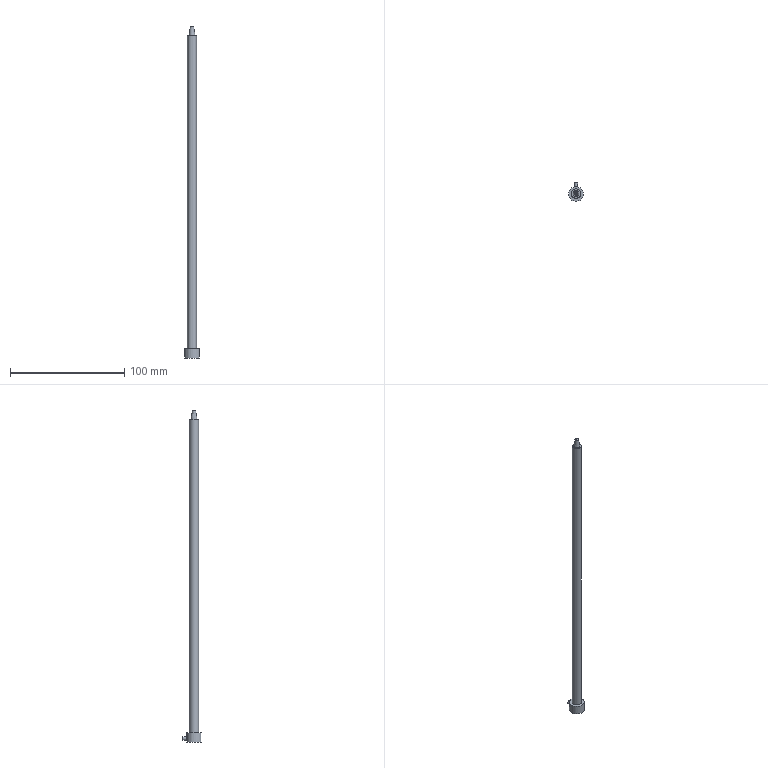Part | STEP file | E108-1-312 | 1 solid | 11 faces | box 13 x 16.5 x 290 mm | volume 14963 mm3 | plane 5 | cylinder 3 | cone 2 | spline 1 | commonest cylinder face diameters 3 x1 8 x1 13 x1
STEP:
#1=CARTESIAN_POINT('',(0.,0.,0.));
#2=DIRECTION('',(0.,0.,1.));
#3=DIRECTION('',(1.,0.,0.));
#4=AXIS2_PLACEMENT_3D('',#1,#2,#3);
#5=CARTESIAN_POINT('',(-4.,0.,282.));
#6=VERTEX_POINT('',#5);
#7=CARTESIAN_POINT('',(4.,0.,282.));
#8=VERTEX_POINT('',#7);
#9=CARTESIAN_POINT('',(0.,0.,282.));
#10=DIRECTION('',(0.,0.,1.));
#11=DIRECTION('',(1.,0.,0.));
#12=AXIS2_PLACEMENT_3D('',#9,#10,#11);
#13=CIRCLE('',#12,4.);
#14=CARTESIAN_POINT('',(0.,0.,100.));
#15=DIRECTION('',(0.,0.,-1.));
#16=DIRECTION('',(-1.,0.,0.));
#17=AXIS2_PLACEMENT_3D('',#14,#15,#16);
#18=CYLINDRICAL_SURFACE('',#17,4.);
#19=CARTESIAN_POINT('',(9.425,-182.));
#20=DIRECTION('',(-1.,0.));
#21=VECTOR('',#20,1.);
#22=LINE('',#19,#21);
#23=(GEOMETRIC_REPRESENTATION_CONTEXT(2)PARAMETRIC_REPRESENTATION_CONTEXT()REPRESENTATION_CONTEXT('',''));
#24=DEFINITIONAL_REPRESENTATION('',(#22),#23);
#25=PCURVE('',#18,#24);
#26=CARTESIAN_POINT('',(0.,0.,282.));
#27=DIRECTION('',(0.,0.,1.));
#28=DIRECTION('',(1.,0.,0.));
#29=AXIS2_PLACEMENT_3D('',#26,#27,#28);
#30=PLANE('',#29);
#31=CARTESIAN_POINT('',(0.,0.));
#32=DIRECTION('',(1.,0.));
#33=AXIS2_PLACEMENT_2D('',#31,#32);
#34=CIRCLE('',#33,4.);
#35=(GEOMETRIC_REPRESENTATION_CONTEXT(2)PARAMETRIC_REPRESENTATION_CONTEXT()REPRESENTATION_CONTEXT('',''));
#36=DEFINITIONAL_REPRESENTATION('',(#34),#35);
#37=PCURVE('',#30,#36);
#38=SURFACE_CURVE('',#13,(#25,#37),.PCURVE_S1.);
#39=EDGE_CURVE('',#6,#8,#38,.T.);
#40=ORIENTED_EDGE('',*,*,#39,.F.);
#41=CARTESIAN_POINT('',(-4.,0.,8.));
#42=VERTEX_POINT('',#41);
#43=CARTESIAN_POINT('',(-4.,0.,282.));
#44=CARTESIAN_POINT('',(-4.,0.,8.));
#45=B_SPLINE_CURVE_WITH_KNOTS('',1,(#43,#44),.UNSPECIFIED.,.F.,.F.,(2,2),(-182.,92.),.PIECEWISE_BEZIER_KNOTS.);
#46=CARTESIAN_POINT('',(6.283,0.));
#47=DIRECTION('',(0.,1.));
#48=VECTOR('',#47,1.);
#49=LINE('',#46,#48);
#50=(GEOMETRIC_REPRESENTATION_CONTEXT(2)PARAMETRIC_REPRESENTATION_CONTEXT()REPRESENTATION_CONTEXT('',''));
#51=DEFINITIONAL_REPRESENTATION('',(#49),#50);
#52=PCURVE('',#18,#51);
#53=CARTESIAN_POINT('',(0.,0.));
#54=DIRECTION('',(0.,1.));
#55=VECTOR('',#54,1.);
#56=LINE('',#53,#55);
#57=(GEOMETRIC_REPRESENTATION_CONTEXT(2)PARAMETRIC_REPRESENTATION_CONTEXT()REPRESENTATION_CONTEXT('',''));
#58=DEFINITIONAL_REPRESENTATION('',(#56),#57);
#59=PCURVE('',#18,#58);
#60=SEAM_CURVE('',#45,(#52,#59),.PCURVE_S1.);
#61=EDGE_CURVE('',#6,#42,#60,.T.);
#62=ORIENTED_EDGE('',*,*,#61,.T.);
#63=CARTESIAN_POINT('',(0.,0.,8.));
#64=DIRECTION('',(0.,0.,1.));
#65=DIRECTION('',(-1.,0.,0.));
#66=AXIS2_PLACEMENT_3D('',#63,#64,#65);
#67=CIRCLE('',#66,4.);
#68=CARTESIAN_POINT('',(6.283,92.));
#69=DIRECTION('',(-1.,0.));
#70=VECTOR('',#69,1.);
#71=LINE('',#68,#70);
#72=(GEOMETRIC_REPRESENTATION_CONTEXT(2)PARAMETRIC_REPRESENTATION_CONTEXT()REPRESENTATION_CONTEXT('',''));
#73=DEFINITIONAL_REPRESENTATION('',(#71),#72);
#74=PCURVE('',#18,#73);
#75=CARTESIAN_POINT('',(0.,0.,8.));
#76=DIRECTION('',(0.,0.,-1.));
#77=DIRECTION('',(1.,0.,0.));
#78=AXIS2_PLACEMENT_3D('',#75,#76,#77);
#79=PLANE('',#78);
#80=CARTESIAN_POINT('',(-4.,0.));
#81=CARTESIAN_POINT('',(-4.,6.928));
#82=CARTESIAN_POINT('',(2.,3.464));
#83=CARTESIAN_POINT('',(8.,0.));
#84=CARTESIAN_POINT('',(2.,-3.464));
#85=CARTESIAN_POINT('',(-4.,-6.928));
#86=CARTESIAN_POINT('',(-4.,0.));
#87=(BOUNDED_CURVE()B_SPLINE_CURVE(2,(#80,#81,#82,#83,#84,#85,#86),.UNSPECIFIED.,.T.,.F.)B_SPLINE_CURVE_WITH_KNOTS((1,2,2,2,2,1),(-2.094,0.,2.094,4.189,6.283,8.378),.UNSPECIFIED.)CURVE()GEOMETRIC_REPRESENTATION_ITEM()RATIONAL_B_SPLINE_CURVE((1.,0.5,1.,0.5,1.,0.5,1.))REPRESENTATION_ITEM(''));
#88=(GEOMETRIC_REPRESENTATION_CONTEXT(2)PARAMETRIC_REPRESENTATION_CONTEXT()REPRESENTATION_CONTEXT('',''));
#89=DEFINITIONAL_REPRESENTATION('',(#87),#88);
#90=PCURVE('',#79,#89);
#91=SURFACE_CURVE('',#67,(#74,#90),.PCURVE_S1.);
#92=EDGE_CURVE('',#42,#42,#91,.T.);
#93=ORIENTED_EDGE('',*,*,#92,.T.);
#94=ORIENTED_EDGE('',*,*,#61,.F.);
#95=CARTESIAN_POINT('',(0.,0.,282.));
#96=DIRECTION('',(0.,0.,1.));
#97=DIRECTION('',(1.,0.,0.));
#98=AXIS2_PLACEMENT_3D('',#95,#96,#97);
#99=CIRCLE('',#98,4.);
#100=CARTESIAN_POINT('',(3.142,-182.));
#101=DIRECTION('',(-1.,0.));
#102=VECTOR('',#101,1.);
#103=LINE('',#100,#102);
#104=(GEOMETRIC_REPRESENTATION_CONTEXT(2)PARAMETRIC_REPRESENTATION_CONTEXT()REPRESENTATION_CONTEXT('',''));
#105=DEFINITIONAL_REPRESENTATION('',(#103),#104);
#106=PCURVE('',#18,#105);
#107=CARTESIAN_POINT('',(0.,0.));
#108=DIRECTION('',(1.,0.));
#109=AXIS2_PLACEMENT_2D('',#107,#108);
#110=CIRCLE('',#109,4.);
#111=(GEOMETRIC_REPRESENTATION_CONTEXT(2)PARAMETRIC_REPRESENTATION_CONTEXT()REPRESENTATION_CONTEXT('',''));
#112=DEFINITIONAL_REPRESENTATION('',(#110),#111);
#113=PCURVE('',#30,#112);
#114=SURFACE_CURVE('',#99,(#106,#113),.PCURVE_S1.);
#115=EDGE_CURVE('',#8,#6,#114,.T.);
#116=ORIENTED_EDGE('',*,*,#115,.F.);
#117=EDGE_LOOP('',(#40,#62,#93,#94,#116));
#118=FACE_BOUND('',#117,.T.);
#119=ADVANCED_FACE('',(#118),#18,.T.);
#120=CARTESIAN_POINT('',(2.553,0.,282.));
#121=VERTEX_POINT('',#120);
#122=CARTESIAN_POINT('',(0.,0.,282.));
#123=DIRECTION('',(0.,0.,1.));
#124=DIRECTION('',(1.,0.,0.));
#125=AXIS2_PLACEMENT_3D('',#122,#123,#124);
#126=CIRCLE('',#125,2.553);
#127=CARTESIAN_POINT('',(0.,0.));
#128=DIRECTION('',(1.,0.));
#129=AXIS2_PLACEMENT_2D('',#127,#128);
#130=CIRCLE('',#129,2.553);
#131=(GEOMETRIC_REPRESENTATION_CONTEXT(2)PARAMETRIC_REPRESENTATION_CONTEXT()REPRESENTATION_CONTEXT('',''));
#132=DEFINITIONAL_REPRESENTATION('',(#130),#131);
#133=PCURVE('',#30,#132);
#134=CARTESIAN_POINT('',(0.,0.,290.));
#135=DIRECTION('',(0.,0.,-1.));
#136=DIRECTION('',(1.,0.,0.));
#137=AXIS2_PLACEMENT_3D('',#134,#135,#136);
#138=CONICAL_SURFACE('',#137,1.5,0.1309);
#139=CARTESIAN_POINT('',(6.283,8.));
#140=DIRECTION('',(-1.,0.));
#141=VECTOR('',#140,1.);
#142=LINE('',#139,#141);
#143=(GEOMETRIC_REPRESENTATION_CONTEXT(2)PARAMETRIC_REPRESENTATION_CONTEXT()REPRESENTATION_CONTEXT('',''));
#144=DEFINITIONAL_REPRESENTATION('',(#142),#143);
#145=PCURVE('',#138,#144);
#146=SURFACE_CURVE('',#126,(#133,#145),.PCURVE_S1.);
#147=EDGE_CURVE('',#121,#121,#146,.T.);
#148=ORIENTED_EDGE('',*,*,#147,.F.);
#149=EDGE_LOOP('',(#148));
#150=FACE_BOUND('',#149,.T.);
#151=ORIENTED_EDGE('',*,*,#115,.T.);
#152=ORIENTED_EDGE('',*,*,#39,.T.);
#153=EDGE_LOOP('',(#151,#152));
#154=FACE_BOUND('',#153,.T.);
#155=ADVANCED_FACE('',(#150,#154),#30,.T.);
#156=CARTESIAN_POINT('',(6.5,0.,0.));
#157=VERTEX_POINT('',#156);
#158=CARTESIAN_POINT('',(-6.5,0.,0.));
#159=VERTEX_POINT('',#158);
#160=CARTESIAN_POINT('',(0.,0.,0.));
#161=DIRECTION('',(0.,0.,-1.));
#162=DIRECTION('',(-1.,0.,0.));
#163=AXIS2_PLACEMENT_3D('',#160,#161,#162);
#164=CIRCLE('',#163,6.5);
#165=CARTESIAN_POINT('',(0.,0.,8.));
#166=DIRECTION('',(0.,0.,-1.));
#167=DIRECTION('',(1.,0.,0.));
#168=AXIS2_PLACEMENT_3D('',#165,#166,#167);
#169=CYLINDRICAL_SURFACE('',#168,6.5);
#170=CARTESIAN_POINT('',(-3.142,8.));
#171=DIRECTION('',(1.,0.));
#172=VECTOR('',#171,1.);
#173=LINE('',#170,#172);
#174=(GEOMETRIC_REPRESENTATION_CONTEXT(2)PARAMETRIC_REPRESENTATION_CONTEXT()REPRESENTATION_CONTEXT('',''));
#175=DEFINITIONAL_REPRESENTATION('',(#173),#174);
#176=PCURVE('',#169,#175);
#177=CARTESIAN_POINT('',(240.,-1000.,0.));
#178=DIRECTION('',(0.,0.,1.));
#179=DIRECTION('',(-1.,0.,0.));
#180=AXIS2_PLACEMENT_3D('',#177,#178,#179);
#181=PLANE('',#180);
#182=CARTESIAN_POINT('',(246.5,-1000.));
#183=CARTESIAN_POINT('',(246.5,-1011.258));
#184=CARTESIAN_POINT('',(236.75,-1005.629));
#185=CARTESIAN_POINT('',(227.,-1000.));
#186=CARTESIAN_POINT('',(236.75,-994.371));
#187=CARTESIAN_POINT('',(246.5,-988.742));
#188=CARTESIAN_POINT('',(246.5,-1000.));
#189=(BOUNDED_CURVE()B_SPLINE_CURVE(2,(#182,#183,#184,#185,#186,#187,#188),.UNSPECIFIED.,.T.,.F.)B_SPLINE_CURVE_WITH_KNOTS((1,2,2,2,2,1),(-2.094,0.,2.094,4.189,6.283,8.378),.UNSPECIFIED.)CURVE()GEOMETRIC_REPRESENTATION_ITEM()RATIONAL_B_SPLINE_CURVE((1.,0.5,1.,0.5,1.,0.5,1.))REPRESENTATION_ITEM(''));
#190=(GEOMETRIC_REPRESENTATION_CONTEXT(2)PARAMETRIC_REPRESENTATION_CONTEXT()REPRESENTATION_CONTEXT('',''));
#191=DEFINITIONAL_REPRESENTATION('',(#189),#190);
#192=PCURVE('',#181,#191);
#193=SURFACE_CURVE('',#164,(#176,#192),.PCURVE_S1.);
#194=EDGE_CURVE('',#157,#159,#193,.T.);
#195=ORIENTED_EDGE('',*,*,#194,.F.);
#196=CARTESIAN_POINT('',(6.5,0.,8.));
#197=VERTEX_POINT('',#196);
#198=CARTESIAN_POINT('',(6.5,0.,8.));
#199=CARTESIAN_POINT('',(6.5,0.,0.));
#200=B_SPLINE_CURVE_WITH_KNOTS('',1,(#198,#199),.UNSPECIFIED.,.F.,.F.,(2,2),(0.,8.),.PIECEWISE_BEZIER_KNOTS.);
#201=CARTESIAN_POINT('',(0.,0.));
#202=DIRECTION('',(0.,1.));
#203=VECTOR('',#202,1.);
#204=LINE('',#201,#203);
#205=(GEOMETRIC_REPRESENTATION_CONTEXT(2)PARAMETRIC_REPRESENTATION_CONTEXT()REPRESENTATION_CONTEXT('',''));
#206=DEFINITIONAL_REPRESENTATION('',(#204),#205);
#207=PCURVE('',#169,#206);
#208=CARTESIAN_POINT('',(6.283,0.));
#209=DIRECTION('',(0.,1.));
#210=VECTOR('',#209,1.);
#211=LINE('',#208,#210);
#212=(GEOMETRIC_REPRESENTATION_CONTEXT(2)PARAMETRIC_REPRESENTATION_CONTEXT()REPRESENTATION_CONTEXT('',''));
#213=DEFINITIONAL_REPRESENTATION('',(#211),#212);
#214=PCURVE('',#169,#213);
#215=SEAM_CURVE('',#200,(#207,#214),.PCURVE_S1.);
#216=EDGE_CURVE('',#197,#157,#215,.T.);
#217=ORIENTED_EDGE('',*,*,#216,.F.);
#218=CARTESIAN_POINT('',(0.,0.,8.));
#219=DIRECTION('',(0.,0.,-1.));
#220=DIRECTION('',(1.,0.,0.));
#221=AXIS2_PLACEMENT_3D('',#218,#219,#220);
#222=CIRCLE('',#221,6.5);
#223=CARTESIAN_POINT('',(0.,0.));
#224=DIRECTION('',(1.,0.));
#225=VECTOR('',#224,1.);
#226=LINE('',#223,#225);
#227=(GEOMETRIC_REPRESENTATION_CONTEXT(2)PARAMETRIC_REPRESENTATION_CONTEXT()REPRESENTATION_CONTEXT('',''));
#228=DEFINITIONAL_REPRESENTATION('',(#226),#227);
#229=PCURVE('',#169,#228);
#230=CARTESIAN_POINT('',(0.,0.));
#231=DIRECTION('',(1.,0.));
#232=AXIS2_PLACEMENT_2D('',#230,#231);
#233=CIRCLE('',#232,6.5);
#234=(GEOMETRIC_REPRESENTATION_CONTEXT(2)PARAMETRIC_REPRESENTATION_CONTEXT()REPRESENTATION_CONTEXT('',''));
#235=DEFINITIONAL_REPRESENTATION('',(#233),#234);
#236=PCURVE('',#79,#235);
#237=SURFACE_CURVE('',#222,(#229,#236),.PCURVE_S1.);
#238=EDGE_CURVE('',#197,#197,#237,.T.);
#239=ORIENTED_EDGE('',*,*,#238,.T.);
#240=ORIENTED_EDGE('',*,*,#216,.T.);
#241=CARTESIAN_POINT('',(0.,0.,0.));
#242=DIRECTION('',(0.,0.,-1.));
#243=DIRECTION('',(-1.,0.,0.));
#244=AXIS2_PLACEMENT_3D('',#241,#242,#243);
#245=CIRCLE('',#244,6.5);
#246=CARTESIAN_POINT('',(3.142,8.));
#247=DIRECTION('',(1.,0.));
#248=VECTOR('',#247,1.);
#249=LINE('',#246,#248);
#250=(GEOMETRIC_REPRESENTATION_CONTEXT(2)PARAMETRIC_REPRESENTATION_CONTEXT()REPRESENTATION_CONTEXT('',''));
#251=DEFINITIONAL_REPRESENTATION('',(#249),#250);
#252=PCURVE('',#169,#251);
#253=CARTESIAN_POINT('',(246.5,-1000.));
#254=CARTESIAN_POINT('',(246.5,-1011.258));
#255=CARTESIAN_POINT('',(236.75,-1005.629));
#256=CARTESIAN_POINT('',(227.,-1000.));
#257=CARTESIAN_POINT('',(236.75,-994.371));
#258=CARTESIAN_POINT('',(246.5,-988.742));
#259=CARTESIAN_POINT('',(246.5,-1000.));
#260=(BOUNDED_CURVE()B_SPLINE_CURVE(2,(#253,#254,#255,#256,#257,#258,#259),.UNSPECIFIED.,.T.,.F.)B_SPLINE_CURVE_WITH_KNOTS((1,2,2,2,2,1),(-2.094,0.,2.094,4.189,6.283,8.378),.UNSPECIFIED.)CURVE()GEOMETRIC_REPRESENTATION_ITEM()RATIONAL_B_SPLINE_CURVE((1.,0.5,1.,0.5,1.,0.5,1.))REPRESENTATION_ITEM(''));
#261=(GEOMETRIC_REPRESENTATION_CONTEXT(2)PARAMETRIC_REPRESENTATION_CONTEXT()REPRESENTATION_CONTEXT('',''));
#262=DEFINITIONAL_REPRESENTATION('',(#260),#261);
#263=PCURVE('',#181,#262);
#264=SURFACE_CURVE('',#245,(#252,#263),.PCURVE_S1.);
#265=EDGE_CURVE('',#159,#157,#264,.T.);
#266=ORIENTED_EDGE('',*,*,#265,.F.);
#267=EDGE_LOOP('',(#195,#217,#239,#240,#266));
#268=FACE_BOUND('',#267,.T.);
#269=CARTESIAN_POINT('',(0.,6.5,1.5));
#270=VERTEX_POINT('',#269);
#271=CARTESIAN_POINT('',(0.,6.5,1.5));
#272=CARTESIAN_POINT('',(0.1654,6.5,1.5));
#273=CARTESIAN_POINT('',(0.3332,6.493,1.528));
#274=CARTESIAN_POINT('',(0.4892,6.482,1.582));
#275=CARTESIAN_POINT('',(0.6451,6.47,1.636));
#276=CARTESIAN_POINT('',(0.7936,6.453,1.717));
#277=CARTESIAN_POINT('',(0.9231,6.434,1.818));
#278=CARTESIAN_POINT('',(1.055,6.415,1.92));
#279=CARTESIAN_POINT('',(1.17,6.394,2.047));
#280=CARTESIAN_POINT('',(1.261,6.377,2.187));
#281=CARTESIAN_POINT('',(1.352,6.358,2.329));
#282=CARTESIAN_POINT('',(1.421,6.343,2.49));
#283=CARTESIAN_POINT('',(1.46,6.334,2.655));
#284=CARTESIAN_POINT('',(1.498,6.325,2.817));
#285=CARTESIAN_POINT('',(1.509,6.322,2.989));
#286=CARTESIAN_POINT('',(1.492,6.326,3.155));
#287=CARTESIAN_POINT('',(1.475,6.33,3.318));
#288=CARTESIAN_POINT('',(1.431,6.341,3.48));
#289=CARTESIAN_POINT('',(1.362,6.356,3.628));
#290=CARTESIAN_POINT('',(1.293,6.37,3.777));
#291=CARTESIAN_POINT('',(1.199,6.39,3.917));
#292=CARTESIAN_POINT('',(1.085,6.409,4.035));
#293=CARTESIAN_POINT('',(0.9695,6.428,4.157));
#294=CARTESIAN_POINT('',(0.8309,6.448,4.26));
#295=CARTESIAN_POINT('',(0.6809,6.464,4.337));
#296=CARTESIAN_POINT('',(0.5305,6.48,4.413));
#297=CARTESIAN_POINT('',(0.3642,6.492,4.465));
#298=CARTESIAN_POINT('',(0.1962,6.497,4.487));
#299=CARTESIAN_POINT('',(0.03191,6.502,4.509));
#300=CARTESIAN_POINT('',(-0.1386,6.501,4.503));
#301=CARTESIAN_POINT('',(-0.3008,6.493,4.47));
#302=CARTESIAN_POINT('',(-0.4611,6.486,4.437));
#303=CARTESIAN_POINT('',(-0.6177,6.472,4.377));
#304=CARTESIAN_POINT('',(-0.7583,6.456,4.294));
#305=CARTESIAN_POINT('',(-0.9011,6.439,4.211));
#306=CARTESIAN_POINT('',(-1.031,6.419,4.102));
#307=CARTESIAN_POINT('',(-1.139,6.399,3.976));
#308=CARTESIAN_POINT('',(-1.249,6.38,3.848));
#309=CARTESIAN_POINT('',(-1.338,6.361,3.699));
#310=CARTESIAN_POINT('',(-1.399,6.348,3.541));
#311=CARTESIAN_POINT('',(-1.46,6.334,3.384));
#312=CARTESIAN_POINT('',(-1.494,6.326,3.214));
#313=CARTESIAN_POINT('',(-1.499,6.325,3.046));
#314=CARTESIAN_POINT('',(-1.504,6.324,2.881));
#315=CARTESIAN_POINT('',(-1.482,6.329,2.714));
#316=CARTESIAN_POINT('',(-1.433,6.34,2.557));
#317=CARTESIAN_POINT('',(-1.385,6.351,2.4));
#318=CARTESIAN_POINT('',(-1.309,6.367,2.25));
#319=CARTESIAN_POINT('',(-1.214,6.386,2.119));
#320=CARTESIAN_POINT('',(-1.116,6.404,1.984));
#321=CARTESIAN_POINT('',(-0.9937,6.425,1.864));
#322=CARTESIAN_POINT('',(-0.8569,6.443,1.769));
#323=CARTESIAN_POINT('',(-0.7182,6.462,1.672));
#324=CARTESIAN_POINT('',(-0.5604,6.478,1.598));
#325=CARTESIAN_POINT('',(-0.3967,6.488,1.553));
#326=CARTESIAN_POINT('',(-0.2682,6.496,1.518));
#327=CARTESIAN_POINT('',(-0.1335,6.5,1.5));
#328=CARTESIAN_POINT('',(0.,6.5,1.5));
#329=B_SPLINE_CURVE_WITH_KNOTS('',3,(#271,#272,#273,#274,#275,#276,#277,#278,#279,#280,#281,#282,#283,#284,#285,#286,#287,#288,#289,#290,#291,#292,#293,#294,#295,#296,#297,#298,#299,#300,#301,#302,#303,#304,#305,#306,#307,#308,#309,#310,#311,#312,#313,#314,#315,#316,#317,#318,#319,#320,#321,#322,#323,#324,#325,#326,#327,#328),.UNSPECIFIED.,.T.,.F.,(1,3,3,3,3,3,3,3,3,3,3,3,3,3,3,3,3,3,3,3,3,1),(-0.04234,0.,0.05275,0.1054,0.159,0.2132,0.2665,0.3187,0.3713,0.4252,0.4793,0.5321,0.5843,0.6373,0.6915,0.7453,0.7978,0.85,0.9034,0.9577,1.,1.053),.UNSPECIFIED.);
#330=CARTESIAN_POINT('',(4.712,6.5));
#331=CARTESIAN_POINT('',(4.718,6.5));
#332=CARTESIAN_POINT('',(4.729,6.497));
#333=CARTESIAN_POINT('',(4.745,6.486));
#334=CARTESIAN_POINT('',(4.762,6.467));
#335=CARTESIAN_POINT('',(4.778,6.44));
#336=CARTESIAN_POINT('',(4.793,6.406));
#337=CARTESIAN_POINT('',(4.809,6.365));
#338=CARTESIAN_POINT('',(4.823,6.317));
#339=CARTESIAN_POINT('',(4.838,6.262));
#340=CARTESIAN_POINT('',(4.851,6.201));
#341=CARTESIAN_POINT('',(4.864,6.135));
#342=CARTESIAN_POINT('',(4.876,6.062));
#343=CARTESIAN_POINT('',(4.888,5.983));
#344=CARTESIAN_POINT('',(4.898,5.9));
#345=CARTESIAN_POINT('',(4.908,5.813));
#346=CARTESIAN_POINT('',(4.916,5.721));
#347=CARTESIAN_POINT('',(4.924,5.625));
#348=CARTESIAN_POINT('',(4.93,5.526));
#349=CARTESIAN_POINT('',(4.936,5.424));
#350=CARTESIAN_POINT('',(4.94,5.321));
#351=CARTESIAN_POINT('',(4.943,5.215));
#352=CARTESIAN_POINT('',(4.945,5.108));
#353=CARTESIAN_POINT('',(4.945,5.));
#354=CARTESIAN_POINT('',(4.945,4.893));
#355=CARTESIAN_POINT('',(4.943,4.787));
#356=CARTESIAN_POINT('',(4.94,4.681));
#357=CARTESIAN_POINT('',(4.936,4.576));
#358=CARTESIAN_POINT('',(4.93,4.474));
#359=CARTESIAN_POINT('',(4.924,4.376));
#360=CARTESIAN_POINT('',(4.916,4.28));
#361=CARTESIAN_POINT('',(4.908,4.188));
#362=CARTESIAN_POINT('',(4.898,4.1));
#363=CARTESIAN_POINT('',(4.888,4.017));
#364=CARTESIAN_POINT('',(4.877,3.939));
#365=CARTESIAN_POINT('',(4.864,3.866));
#366=CARTESIAN_POINT('',(4.851,3.799));
#367=CARTESIAN_POINT('',(4.838,3.738));
#368=CARTESIAN_POINT('',(4.824,3.683));
#369=CARTESIAN_POINT('',(4.809,3.635));
#370=CARTESIAN_POINT('',(4.793,3.594));
#371=CARTESIAN_POINT('',(4.778,3.56));
#372=CARTESIAN_POINT('',(4.762,3.533));
#373=CARTESIAN_POINT('',(4.745,3.514));
#374=CARTESIAN_POINT('',(4.729,3.503));
#375=CARTESIAN_POINT('',(4.713,3.499));
#376=CARTESIAN_POINT('',(4.696,3.503));
#377=CARTESIAN_POINT('',(4.679,3.514));
#378=CARTESIAN_POINT('',(4.663,3.533));
#379=CARTESIAN_POINT('',(4.647,3.56));
#380=CARTESIAN_POINT('',(4.632,3.594));
#381=CARTESIAN_POINT('',(4.616,3.635));
#382=CARTESIAN_POINT('',(4.601,3.683));
#383=CARTESIAN_POINT('',(4.587,3.737));
#384=CARTESIAN_POINT('',(4.574,3.798));
#385=CARTESIAN_POINT('',(4.561,3.865));
#386=CARTESIAN_POINT('',(4.548,3.938));
#387=CARTESIAN_POINT('',(4.537,4.016));
#388=CARTESIAN_POINT('',(4.527,4.099));
#389=CARTESIAN_POINT('',(4.517,4.187));
#390=CARTESIAN_POINT('',(4.508,4.279));
#391=CARTESIAN_POINT('',(4.501,4.375));
#392=CARTESIAN_POINT('',(4.494,4.473));
#393=CARTESIAN_POINT('',(4.489,4.575));
#394=CARTESIAN_POINT('',(4.485,4.679));
#395=CARTESIAN_POINT('',(4.482,4.785));
#396=CARTESIAN_POINT('',(4.48,4.892));
#397=CARTESIAN_POINT('',(4.479,4.999));
#398=CARTESIAN_POINT('',(4.48,5.106));
#399=CARTESIAN_POINT('',(4.482,5.213));
#400=CARTESIAN_POINT('',(4.485,5.319));
#401=CARTESIAN_POINT('',(4.489,5.423));
#402=CARTESIAN_POINT('',(4.494,5.524));
#403=CARTESIAN_POINT('',(4.501,5.624));
#404=CARTESIAN_POINT('',(4.508,5.72));
#405=CARTESIAN_POINT('',(4.517,5.812));
#406=CARTESIAN_POINT('',(4.526,5.899));
#407=CARTESIAN_POINT('',(4.537,5.982));
#408=CARTESIAN_POINT('',(4.548,6.061));
#409=CARTESIAN_POINT('',(4.56,6.134));
#410=CARTESIAN_POINT('',(4.573,6.201));
#411=CARTESIAN_POINT('',(4.587,6.262));
#412=CARTESIAN_POINT('',(4.601,6.316));
#413=CARTESIAN_POINT('',(4.616,6.364));
#414=CARTESIAN_POINT('',(4.631,6.406));
#415=CARTESIAN_POINT('',(4.647,6.44));
#416=CARTESIAN_POINT('',(4.663,6.466));
#417=CARTESIAN_POINT('',(4.679,6.486));
#418=CARTESIAN_POINT('',(4.696,6.497));
#419=CARTESIAN_POINT('',(4.707,6.5));
#420=CARTESIAN_POINT('',(4.712,6.5));
#421=B_SPLINE_CURVE_WITH_KNOTS('',3,(#330,#331,#332,#333,#334,#335,#336,#337,#338,#339,#340,#341,#342,#343,#344,#345,#346,#347,#348,#349,#350,#351,#352,#353,#354,#355,#356,#357,#358,#359,#360,#361,#362,#363,#364,#365,#366,#367,#368,#369,#370,#371,#372,#373,#374,#375,#376,#377,#378,#379,#380,#381,#382,#383,#384,#385,#386,#387,#388,#389,#390,#391,#392,#393,#394,#395,#396,#397,#398,#399,#400,#401,#402,#403,#404,#405,#406,#407,#408,#409,#410,#411,#412,#413,#414,#415,#416,#417,#418,#419,#420),.UNSPECIFIED.,.T.,.F.,(4,1,1,1,1,1,1,1,1,1,1,1,1,1,1,1,1,1,1,1,1,1,1,1,1,1,1,1,1,1,1,1,1,1,1,1,1,1,1,1,1,1,1,1,1,1,1,1,1,1,1,1,1,1,1,1,1,1,1,1,1,1,1,1,1,1,1,1,1,1,1,1,1,1,1,1,1,1,1,1,1,1,1,1,1,1,1,1,4),(0.,0.01136,0.02273,0.03409,0.04545,0.05682,0.06818,0.07955,0.09091,0.1023,0.1136,0.125,0.1364,0.1477,0.1591,0.1705,0.1818,0.1932,0.2045,0.2159,0.2273,0.2386,0.25,0.2614,0.2727,0.2841,0.2955,0.3068,0.3182,0.3295,0.3409,0.3523,0.3636,0.375,0.3864,0.3977,0.4091,0.4205,0.4318,0.4432,0.4545,0.4659,0.4773,0.4886,0.5,0.5114,0.5227,0.5341,0.5455,0.5568,0.5682,0.5795,0.5909,0.6023,0.6136,0.625,0.6364,0.6477,0.6591,0.6705,0.6818,0.6932,0.7045,0.7159,0.7273,0.7386,0.75,0.7614,0.7727,0.7841,0.7955,0.8068,0.8182,0.8295,0.8409,0.8523,0.8636,0.875,0.8864,0.8977,0.9091,0.9205,0.9318,0.9432,0.9545,0.9659,0.9773,0.9886,1.),.QUASI_UNIFORM_KNOTS.);
#422=(GEOMETRIC_REPRESENTATION_CONTEXT(2)PARAMETRIC_REPRESENTATION_CONTEXT()REPRESENTATION_CONTEXT('',''));
#423=DEFINITIONAL_REPRESENTATION('',(#421),#422);
#424=PCURVE('',#169,#423);
#425=CARTESIAN_POINT('',(0.,2.,3.));
#426=DIRECTION('',(0.,1.,0.));
#427=DIRECTION('',(0.,0.,-1.));
#428=AXIS2_PLACEMENT_3D('',#425,#426,#427);
#429=CYLINDRICAL_SURFACE('',#428,1.5);
#430=CARTESIAN_POINT('',(6.283,4.5));
#431=CARTESIAN_POINT('',(6.259,4.5));
#432=CARTESIAN_POINT('',(6.212,4.499));
#433=CARTESIAN_POINT('',(6.14,4.497));
#434=CARTESIAN_POINT('',(6.068,4.492));
#435=CARTESIAN_POINT('',(5.997,4.486));
#436=CARTESIAN_POINT('',(5.926,4.479));
#437=CARTESIAN_POINT('',(5.854,4.47));
#438=CARTESIAN_POINT('',(5.783,4.46));
#439=CARTESIAN_POINT('',(5.711,4.449));
#440=CARTESIAN_POINT('',(5.64,4.438));
#441=CARTESIAN_POINT('',(5.569,4.425));
#442=CARTESIAN_POINT('',(5.498,4.413));
#443=CARTESIAN_POINT('',(5.427,4.4));
#444=CARTESIAN_POINT('',(5.355,4.388));
#445=CARTESIAN_POINT('',(5.284,4.376));
#446=CARTESIAN_POINT('',(5.213,4.365));
#447=CARTESIAN_POINT('',(5.142,4.355));
#448=CARTESIAN_POINT('',(5.07,4.346));
#449=CARTESIAN_POINT('',(4.999,4.338));
#450=CARTESIAN_POINT('',(4.928,4.332));
#451=CARTESIAN_POINT('',(4.856,4.328));
#452=CARTESIAN_POINT('',(4.784,4.325));
#453=CARTESIAN_POINT('',(4.713,4.324));
#454=CARTESIAN_POINT('',(4.641,4.325));
#455=CARTESIAN_POINT('',(4.57,4.328));
#456=CARTESIAN_POINT('',(4.498,4.332));
#457=CARTESIAN_POINT('',(4.426,4.339));
#458=CARTESIAN_POINT('',(4.355,4.346));
#459=CARTESIAN_POINT('',(4.283,4.355));
#460=CARTESIAN_POINT('',(4.212,4.365));
#461=CARTESIAN_POINT('',(4.141,4.376));
#462=CARTESIAN_POINT('',(4.07,4.388));
#463=CARTESIAN_POINT('',(3.998,4.4));
#464=CARTESIAN_POINT('',(3.927,4.413));
#465=CARTESIAN_POINT('',(3.856,4.425));
#466=CARTESIAN_POINT('',(3.785,4.437));
#467=CARTESIAN_POINT('',(3.714,4.449));
#468=CARTESIAN_POINT('',(3.642,4.46));
#469=CARTESIAN_POINT('',(3.571,4.47));
#470=CARTESIAN_POINT('',(3.5,4.479));
#471=CARTESIAN_POINT('',(3.428,4.486));
#472=CARTESIAN_POINT('',(3.357,4.492));
#473=CARTESIAN_POINT('',(3.285,4.497));
#474=CARTESIAN_POINT('',(3.214,4.499));
#475=CARTESIAN_POINT('',(3.142,4.5));
#476=CARTESIAN_POINT('',(3.07,4.499));
#477=CARTESIAN_POINT('',(2.999,4.497));
#478=CARTESIAN_POINT('',(2.927,4.492));
#479=CARTESIAN_POINT('',(2.856,4.486));
#480=CARTESIAN_POINT('',(2.784,4.479));
#481=CARTESIAN_POINT('',(2.713,4.47));
#482=CARTESIAN_POINT('',(2.641,4.46));
#483=CARTESIAN_POINT('',(2.57,4.449));
#484=CARTESIAN_POINT('',(2.499,4.438));
#485=CARTESIAN_POINT('',(2.428,4.425));
#486=CARTESIAN_POINT('',(2.357,4.413));
#487=CARTESIAN_POINT('',(2.285,4.4));
#488=CARTESIAN_POINT('',(2.215,4.388));
#489=CARTESIAN_POINT('',(2.143,4.376));
#490=CARTESIAN_POINT('',(2.072,4.365));
#491=CARTESIAN_POINT('',(2.,4.355));
#492=CARTESIAN_POINT('',(1.929,4.346));
#493=CARTESIAN_POINT('',(1.858,4.339));
#494=CARTESIAN_POINT('',(1.786,4.332));
#495=CARTESIAN_POINT('',(1.715,4.328));
#496=CARTESIAN_POINT('',(1.643,4.325));
#497=CARTESIAN_POINT('',(1.572,4.324));
#498=CARTESIAN_POINT('',(1.5,4.325));
#499=CARTESIAN_POINT('',(1.428,4.328));
#500=CARTESIAN_POINT('',(1.357,4.332));
#501=CARTESIAN_POINT('',(1.285,4.338));
#502=CARTESIAN_POINT('',(1.214,4.346));
#503=CARTESIAN_POINT('',(1.142,4.355));
#504=CARTESIAN_POINT('',(1.071,4.365));
#505=CARTESIAN_POINT('',(0.9995,4.376));
#506=CARTESIAN_POINT('',(0.9286,4.388));
#507=CARTESIAN_POINT('',(0.8575,4.4));
#508=CARTESIAN_POINT('',(0.7862,4.413));
#509=CARTESIAN_POINT('',(0.7149,4.425));
#510=CARTESIAN_POINT('',(0.6436,4.437));
#511=CARTESIAN_POINT('',(0.5728,4.449));
#512=CARTESIAN_POINT('',(0.5015,4.46));
#513=CARTESIAN_POINT('',(0.43,4.47));
#514=CARTESIAN_POINT('',(0.3585,4.479));
#515=CARTESIAN_POINT('',(0.2872,4.486));
#516=CARTESIAN_POINT('',(0.2157,4.492));
#517=CARTESIAN_POINT('',(0.1438,4.497));
#518=CARTESIAN_POINT('',(0.07178,4.499));
#519=CARTESIAN_POINT('',(0.02388,4.5));
#520=CARTESIAN_POINT('',(0.,4.5));
#521=B_SPLINE_CURVE_WITH_KNOTS('',3,(#430,#431,#432,#433,#434,#435,#436,#437,#438,#439,#440,#441,#442,#443,#444,#445,#446,#447,#448,#449,#450,#451,#452,#453,#454,#455,#456,#457,#458,#459,#460,#461,#462,#463,#464,#465,#466,#467,#468,#469,#470,#471,#472,#473,#474,#475,#476,#477,#478,#479,#480,#481,#482,#483,#484,#485,#486,#487,#488,#489,#490,#491,#492,#493,#494,#495,#496,#497,#498,#499,#500,#501,#502,#503,#504,#505,#506,#507,#508,#509,#510,#511,#512,#513,#514,#515,#516,#517,#518,#519,#520),.UNSPECIFIED.,.F.,.F.,(4,1,1,1,1,1,1,1,1,1,1,1,1,1,1,1,1,1,1,1,1,1,1,1,1,1,1,1,1,1,1,1,1,1,1,1,1,1,1,1,1,1,1,1,1,1,1,1,1,1,1,1,1,1,1,1,1,1,1,1,1,1,1,1,1,1,1,1,1,1,1,1,1,1,1,1,1,1,1,1,1,1,1,1,1,1,1,1,4),(0.,0.01136,0.02273,0.03409,0.04545,0.05682,0.06818,0.07955,0.09091,0.1023,0.1136,0.125,0.1364,0.1477,0.1591,0.1705,0.1818,0.1932,0.2045,0.2159,0.2273,0.2386,0.25,0.2614,0.2727,0.2841,0.2955,0.3068,0.3182,0.3295,0.3409,0.3523,0.3636,0.375,0.3864,0.3977,0.4091,0.4205,0.4318,0.4432,0.4545,0.4659,0.4773,0.4886,0.5,0.5114,0.5227,0.5341,0.5455,0.5568,0.5682,0.5795,0.5909,0.6023,0.6136,0.625,0.6364,0.6477,0.6591,0.6705,0.6818,0.6932,0.7045,0.7159,0.7273,0.7386,0.75,0.7614,0.7727,0.7841,0.7955,0.8068,0.8182,0.8295,0.8409,0.8523,0.8636,0.875,0.8864,0.8977,0.9091,0.9205,0.9318,0.9432,0.9545,0.9659,0.9773,0.9886,1.),.QUASI_UNIFORM_KNOTS.);
#522=(GEOMETRIC_REPRESENTATION_CONTEXT(2)PARAMETRIC_REPRESENTATION_CONTEXT()REPRESENTATION_CONTEXT('',''));
#523=DEFINITIONAL_REPRESENTATION('',(#521),#522);
#524=PCURVE('',#429,#523);
#525=SURFACE_CURVE('',#329,(#424,#524),.PCURVE_S1.);
#526=EDGE_CURVE('',#270,#270,#525,.T.);
#527=ORIENTED_EDGE('',*,*,#526,.T.);
#528=EDGE_LOOP('',(#527));
#529=FACE_BOUND('',#528,.T.);
#530=ADVANCED_FACE('',(#268,#529),#169,.T.);
#531=ORIENTED_EDGE('',*,*,#92,.F.);
#532=EDGE_LOOP('',(#531));
#533=FACE_BOUND('',#532,.T.);
#534=ORIENTED_EDGE('',*,*,#238,.F.);
#535=EDGE_LOOP('',(#534));
#536=FACE_BOUND('',#535,.T.);
#537=ADVANCED_FACE('',(#533,#536),#79,.F.);
#538=ORIENTED_EDGE('',*,*,#265,.T.);
#539=ORIENTED_EDGE('',*,*,#194,.T.);
#540=EDGE_LOOP('',(#538,#539));
#541=FACE_BOUND('',#540,.T.);
#542=ADVANCED_FACE('',(#541),#181,.F.);
#543=CARTESIAN_POINT('',(0.,10.,1.75));
#544=VERTEX_POINT('',#543);
#545=CARTESIAN_POINT('',(0.,10.,3.));
#546=DIRECTION('',(0.,1.,0.));
#547=DIRECTION('',(0.,0.,-1.));
#548=AXIS2_PLACEMENT_3D('',#545,#546,#547);
#549=CIRCLE('',#548,1.25);
#550=CARTESIAN_POINT('',(0.,10.,3.));
#551=DIRECTION('',(0.,1.,0.));
#552=DIRECTION('',(0.,0.,-1.));
#553=AXIS2_PLACEMENT_3D('',#550,#551,#552);
#554=PLANE('',#553);
#555=CARTESIAN_POINT('',(0.,0.));
#556=DIRECTION('',(1.,0.));
#557=AXIS2_PLACEMENT_2D('',#555,#556);
#558=CIRCLE('',#557,1.25);
#559=(GEOMETRIC_REPRESENTATION_CONTEXT(2)PARAMETRIC_REPRESENTATION_CONTEXT()REPRESENTATION_CONTEXT('',''));
#560=DEFINITIONAL_REPRESENTATION('',(#558),#559);
#561=PCURVE('',#554,#560);
#562=CARTESIAN_POINT('',(0.,9.75,3.));
#563=DIRECTION('',(0.,-1.,0.));
#564=DIRECTION('',(0.,0.,1.));
#565=AXIS2_PLACEMENT_3D('',#562,#563,#564);
#566=CONICAL_SURFACE('',#565,1.5,0.7854);
#567=CARTESIAN_POINT('',(9.425,-0.25));
#568=DIRECTION('',(-1.,0.));
#569=VECTOR('',#568,1.);
#570=LINE('',#567,#569);
#571=(GEOMETRIC_REPRESENTATION_CONTEXT(2)PARAMETRIC_REPRESENTATION_CONTEXT()REPRESENTATION_CONTEXT('',''));
#572=DEFINITIONAL_REPRESENTATION('',(#570),#571);
#573=PCURVE('',#566,#572);
#574=SURFACE_CURVE('',#549,(#561,#573),.PCURVE_S1.);
#575=EDGE_CURVE('',#544,#544,#574,.T.);
#576=ORIENTED_EDGE('',*,*,#575,.T.);
#577=EDGE_LOOP('',(#576));
#578=FACE_BOUND('',#577,.T.);
#579=ADVANCED_FACE('',(#578),#554,.T.);
#580=ORIENTED_EDGE('',*,*,#575,.F.);
#581=CARTESIAN_POINT('',(0.,9.75,1.5));
#582=VERTEX_POINT('',#581);
#583=CARTESIAN_POINT('',(0.,10.,1.75));
#584=CARTESIAN_POINT('',(0.,9.75,1.5));
#585=B_SPLINE_CURVE_WITH_KNOTS('',1,(#583,#584),.UNSPECIFIED.,.F.,.F.,(2,2),(-0.3536,0.),.PIECEWISE_BEZIER_KNOTS.);
#586=CARTESIAN_POINT('',(9.425,0.));
#587=DIRECTION('',(0.,1.));
#588=VECTOR('',#587,1.);
#589=LINE('',#586,#588);
#590=(GEOMETRIC_REPRESENTATION_CONTEXT(2)PARAMETRIC_REPRESENTATION_CONTEXT()REPRESENTATION_CONTEXT('',''));
#591=DEFINITIONAL_REPRESENTATION('',(#589),#590);
#592=PCURVE('',#566,#591);
#593=CARTESIAN_POINT('',(3.142,0.));
#594=DIRECTION('',(0.,1.));
#595=VECTOR('',#594,1.);
#596=LINE('',#593,#595);
#597=(GEOMETRIC_REPRESENTATION_CONTEXT(2)PARAMETRIC_REPRESENTATION_CONTEXT()REPRESENTATION_CONTEXT('',''));
#598=DEFINITIONAL_REPRESENTATION('',(#596),#597);
#599=PCURVE('',#566,#598);
#600=SEAM_CURVE('',#585,(#592,#599),.PCURVE_S1.);
#601=EDGE_CURVE('',#544,#582,#600,.T.);
#602=ORIENTED_EDGE('',*,*,#601,.T.);
#603=CARTESIAN_POINT('',(0.,9.75,3.));
#604=DIRECTION('',(0.,-1.,0.));
#605=DIRECTION('',(0.,0.,-1.));
#606=AXIS2_PLACEMENT_3D('',#603,#604,#605);
#607=CIRCLE('',#606,1.5);
#608=CARTESIAN_POINT('',(3.142,0.));
#609=DIRECTION('',(1.,0.));
#610=VECTOR('',#609,1.);
#611=LINE('',#608,#610);
#612=(GEOMETRIC_REPRESENTATION_CONTEXT(2)PARAMETRIC_REPRESENTATION_CONTEXT()REPRESENTATION_CONTEXT('',''));
#613=DEFINITIONAL_REPRESENTATION('',(#611),#612);
#614=PCURVE('',#566,#613);
#615=CARTESIAN_POINT('',(6.283,7.75));
#616=DIRECTION('',(-1.,0.));
#617=VECTOR('',#616,1.);
#618=LINE('',#615,#617);
#619=(GEOMETRIC_REPRESENTATION_CONTEXT(2)PARAMETRIC_REPRESENTATION_CONTEXT()REPRESENTATION_CONTEXT('',''));
#620=DEFINITIONAL_REPRESENTATION('',(#618),#619);
#621=PCURVE('',#429,#620);
#622=SURFACE_CURVE('',#607,(#614,#621),.PCURVE_S1.);
#623=EDGE_CURVE('',#582,#582,#622,.T.);
#624=ORIENTED_EDGE('',*,*,#623,.F.);
#625=ORIENTED_EDGE('',*,*,#601,.F.);
#626=EDGE_LOOP('',(#580,#602,#624,#625));
#627=FACE_BOUND('',#626,.T.);
#628=ADVANCED_FACE('',(#627),#566,.T.);
#629=ORIENTED_EDGE('',*,*,#526,.F.);
#630=CARTESIAN_POINT('',(0.,6.5,1.5));
#631=CARTESIAN_POINT('',(0.,9.75,1.5));
#632=B_SPLINE_CURVE_WITH_KNOTS('',1,(#630,#631),.UNSPECIFIED.,.F.,.F.,(2,2),(4.5,7.75),.PIECEWISE_BEZIER_KNOTS.);
#633=CARTESIAN_POINT('',(6.283,0.));
#634=DIRECTION('',(0.,1.));
#635=VECTOR('',#634,1.);
#636=LINE('',#633,#635);
#637=(GEOMETRIC_REPRESENTATION_CONTEXT(2)PARAMETRIC_REPRESENTATION_CONTEXT()REPRESENTATION_CONTEXT('',''));
#638=DEFINITIONAL_REPRESENTATION('',(#636),#637);
#639=PCURVE('',#429,#638);
#640=CARTESIAN_POINT('',(0.,0.));
#641=DIRECTION('',(0.,1.));
#642=VECTOR('',#641,1.);
#643=LINE('',#640,#642);
#644=(GEOMETRIC_REPRESENTATION_CONTEXT(2)PARAMETRIC_REPRESENTATION_CONTEXT()REPRESENTATION_CONTEXT('',''));
#645=DEFINITIONAL_REPRESENTATION('',(#643),#644);
#646=PCURVE('',#429,#645);
#647=SEAM_CURVE('',#632,(#639,#646),.PCURVE_S1.);
#648=EDGE_CURVE('',#270,#582,#647,.T.);
#649=ORIENTED_EDGE('',*,*,#648,.T.);
#650=ORIENTED_EDGE('',*,*,#623,.T.);
#651=ORIENTED_EDGE('',*,*,#648,.F.);
#652=EDGE_LOOP('',(#629,#649,#650,#651));
#653=FACE_BOUND('',#652,.T.);
#654=ADVANCED_FACE('',(#653),#429,.T.);
#655=CARTESIAN_POINT('',(0.623,0.,290.));
#656=VERTEX_POINT('',#655);
#657=CARTESIAN_POINT('',(0.,0.,290.));
#658=DIRECTION('',(0.,0.,1.));
#659=DIRECTION('',(1.,0.,0.));
#660=AXIS2_PLACEMENT_3D('',#657,#658,#659);
#661=CIRCLE('',#660,0.623);
#662=CARTESIAN_POINT('',(0.,0.,290.));
#663=DIRECTION('',(0.,0.,1.));
#664=DIRECTION('',(1.,0.,0.));
#665=AXIS2_PLACEMENT_3D('',#662,#663,#664);
#666=PLANE('',#665);
#667=CARTESIAN_POINT('',(0.,0.));
#668=DIRECTION('',(1.,0.));
#669=AXIS2_PLACEMENT_2D('',#667,#668);
#670=CIRCLE('',#669,0.623);
#671=(GEOMETRIC_REPRESENTATION_CONTEXT(2)PARAMETRIC_REPRESENTATION_CONTEXT()REPRESENTATION_CONTEXT('',''));
#672=DEFINITIONAL_REPRESENTATION('',(#670),#671);
#673=PCURVE('',#666,#672);
#674=CARTESIAN_POINT('',(0.623,0.,290.));
#675=CARTESIAN_POINT('',(0.623,1.246,290.));
#676=CARTESIAN_POINT('',(-0.623,1.246,290.));
#677=CARTESIAN_POINT('',(-0.623,0.,290.));
#678=CARTESIAN_POINT('',(-0.623,-1.246,290.));
#679=CARTESIAN_POINT('',(0.623,-1.246,290.));
#680=CARTESIAN_POINT('',(0.623,0.,290.));
#681=CARTESIAN_POINT('',(1.15,0.,290.));
#682=CARTESIAN_POINT('',(1.15,2.299,290.));
#683=CARTESIAN_POINT('',(-1.15,2.299,290.));
#684=CARTESIAN_POINT('',(-1.15,0.,290.));
#685=CARTESIAN_POINT('',(-1.15,-2.299,290.));
#686=CARTESIAN_POINT('',(1.15,-2.299,290.));
#687=CARTESIAN_POINT('',(1.15,0.,290.));
#688=CARTESIAN_POINT('',(1.546,0.,289.653));
#689=CARTESIAN_POINT('',(1.546,3.091,289.653));
#690=CARTESIAN_POINT('',(-1.546,3.091,289.653));
#691=CARTESIAN_POINT('',(-1.546,0.,289.653));
#692=CARTESIAN_POINT('',(-1.546,-3.091,289.653));
#693=CARTESIAN_POINT('',(1.546,-3.091,289.653));
#694=CARTESIAN_POINT('',(1.546,0.,289.653));
#695=CARTESIAN_POINT('',(1.614,0.,289.131));
#696=CARTESIAN_POINT('',(1.614,3.229,289.131));
#697=CARTESIAN_POINT('',(-1.614,3.229,289.131));
#698=CARTESIAN_POINT('',(-1.614,0.,289.131));
#699=CARTESIAN_POINT('',(-1.614,-3.229,289.131));
#700=CARTESIAN_POINT('',(1.614,-3.229,289.131));
#701=CARTESIAN_POINT('',(1.614,0.,289.131));
#702=(BOUNDED_SURFACE()B_SPLINE_SURFACE(3,3,((#674,#675,#676,#677,#678,#679,#680),(#681,#682,#683,#684,#685,#686,#687),(#688,#689,#690,#691,#692,#693,#694),(#695,#696,#697,#698,#699,#700,#701)),.UNSPECIFIED.,.F.,.T.,.F.)B_SPLINE_SURFACE_WITH_KNOTS((4,4),(1,3,3,3,1),(0.,1.),(-0.5,0.,0.5,1.,1.5),.UNSPECIFIED.)GEOMETRIC_REPRESENTATION_ITEM()RATIONAL_B_SPLINE_SURFACE(((1.,0.3333,0.3333,1.,0.3333,0.3333,1.),(0.8346,0.2782,0.2782,0.8346,0.2782,0.2782,0.8346),(0.8346,0.2782,0.2782,0.8346,0.2782,0.2782,0.8346),(1.,0.3333,0.3333,1.,0.3333,0.3333,1.)))REPRESENTATION_ITEM('')SURFACE());
#703=CARTESIAN_POINT('',(0.,0.));
#704=CARTESIAN_POINT('',(0.,0.02352));
#705=CARTESIAN_POINT('',(0.,0.06491));
#706=CARTESIAN_POINT('',(0.,0.1146));
#707=CARTESIAN_POINT('',(0.,0.1575));
#708=CARTESIAN_POINT('',(0.,0.196));
#709=CARTESIAN_POINT('',(0.,0.2322));
#710=CARTESIAN_POINT('',(0.,0.2678));
#711=CARTESIAN_POINT('',(0.,0.304));
#712=CARTESIAN_POINT('',(0.,0.3425));
#713=CARTESIAN_POINT('',(0.,0.3856));
#714=CARTESIAN_POINT('',(0.,0.4343));
#715=CARTESIAN_POINT('',(0.,0.5));
#716=CARTESIAN_POINT('',(0.,0.5657));
#717=CARTESIAN_POINT('',(0.,0.6144));
#718=CARTESIAN_POINT('',(0.,0.6575));
#719=CARTESIAN_POINT('',(0.,0.696));
#720=CARTESIAN_POINT('',(0.,0.7322));
#721=CARTESIAN_POINT('',(0.,0.7678));
#722=CARTESIAN_POINT('',(0.,0.804));
#723=CARTESIAN_POINT('',(0.,0.8425));
#724=CARTESIAN_POINT('',(0.,0.8854));
#725=CARTESIAN_POINT('',(0.,0.9351));
#726=CARTESIAN_POINT('',(0.,0.9765));
#727=CARTESIAN_POINT('',(0.,1.));
#728=B_SPLINE_CURVE_WITH_KNOTS('',3,(#703,#704,#705,#706,#707,#708,#709,#710,#711,#712,#713,#714,#715,#716,#717,#718,#719,#720,#721,#722,#723,#724,#725,#726,#727),.UNSPECIFIED.,.F.,.F.,(4,1,1,1,1,1,1,1,1,1,1,1,1,1,1,1,1,1,1,1,1,1,4),(0.,0.2856,0.5712,0.8568,1.142,1.428,1.714,1.999,2.285,2.57,2.856,3.142,3.427,3.713,3.998,4.284,4.57,4.855,5.141,5.426,5.712,5.998,6.283),.QUASI_UNIFORM_KNOTS.);
#729=(GEOMETRIC_REPRESENTATION_CONTEXT(2)PARAMETRIC_REPRESENTATION_CONTEXT()REPRESENTATION_CONTEXT('',''));
#730=DEFINITIONAL_REPRESENTATION('',(#728),#729);
#731=PCURVE('',#702,#730);
#732=SURFACE_CURVE('',#661,(#673,#731),.PCURVE_S1.);
#733=EDGE_CURVE('',#656,#656,#732,.T.);
#734=ORIENTED_EDGE('',*,*,#733,.T.);
#735=EDGE_LOOP('',(#734));
#736=FACE_BOUND('',#735,.T.);
#737=ADVANCED_FACE('',(#736),#666,.T.);
#738=ORIENTED_EDGE('',*,*,#733,.F.);
#739=CARTESIAN_POINT('',(1.614,0.,289.131));
#740=VERTEX_POINT('',#739);
#741=CARTESIAN_POINT('',(0.623,0.,290.));
#742=CARTESIAN_POINT('',(1.15,0.,290.));
#743=CARTESIAN_POINT('',(1.546,0.,289.653));
#744=CARTESIAN_POINT('',(1.614,0.,289.131));
#745=(BOUNDED_CURVE()B_SPLINE_CURVE(3,(#741,#742,#743,#744),.UNSPECIFIED.,.F.,.F.)B_SPLINE_CURVE_WITH_KNOTS((4,4),(0.,1.),.PIECEWISE_BEZIER_KNOTS.)CURVE()GEOMETRIC_REPRESENTATION_ITEM()RATIONAL_B_SPLINE_CURVE((1.,0.8346,0.8346,1.))REPRESENTATION_ITEM(''));
#746=CARTESIAN_POINT('',(0.,0.));
#747=DIRECTION('',(1.,0.));
#748=VECTOR('',#747,1.);
#749=LINE('',#746,#748);
#750=(GEOMETRIC_REPRESENTATION_CONTEXT(2)PARAMETRIC_REPRESENTATION_CONTEXT()REPRESENTATION_CONTEXT('',''));
#751=DEFINITIONAL_REPRESENTATION('',(#749),#750);
#752=PCURVE('',#702,#751);
#753=CARTESIAN_POINT('',(0.,1.));
#754=DIRECTION('',(1.,0.));
#755=VECTOR('',#754,1.);
#756=LINE('',#753,#755);
#757=(GEOMETRIC_REPRESENTATION_CONTEXT(2)PARAMETRIC_REPRESENTATION_CONTEXT()REPRESENTATION_CONTEXT('',''));
#758=DEFINITIONAL_REPRESENTATION('',(#756),#757);
#759=PCURVE('',#702,#758);
#760=SEAM_CURVE('',#745,(#752,#759),.PCURVE_S1.);
#761=EDGE_CURVE('',#656,#740,#760,.T.);
#762=ORIENTED_EDGE('',*,*,#761,.T.);
#763=CARTESIAN_POINT('',(0.,0.,289.131));
#764=DIRECTION('',(0.,0.,-1.));
#765=DIRECTION('',(1.,0.,0.));
#766=AXIS2_PLACEMENT_3D('',#763,#764,#765);
#767=CIRCLE('',#766,1.614);
#768=CARTESIAN_POINT('',(1.,1.));
#769=CARTESIAN_POINT('',(1.,0.9765));
#770=CARTESIAN_POINT('',(1.,0.9351));
#771=CARTESIAN_POINT('',(1.,0.8854));
#772=CARTESIAN_POINT('',(1.,0.8425));
#773=CARTESIAN_POINT('',(1.,0.804));
#774=CARTESIAN_POINT('',(1.,0.7678));
#775=CARTESIAN_POINT('',(1.,0.7322));
#776=CARTESIAN_POINT('',(1.,0.696));
#777=CARTESIAN_POINT('',(1.,0.6575));
#778=CARTESIAN_POINT('',(1.,0.6144));
#779=CARTESIAN_POINT('',(1.,0.5657));
#780=CARTESIAN_POINT('',(1.,0.5));
#781=CARTESIAN_POINT('',(1.,0.4343));
#782=CARTESIAN_POINT('',(1.,0.3856));
#783=CARTESIAN_POINT('',(1.,0.3425));
#784=CARTESIAN_POINT('',(1.,0.304));
#785=CARTESIAN_POINT('',(1.,0.2678));
#786=CARTESIAN_POINT('',(1.,0.2322));
#787=CARTESIAN_POINT('',(1.,0.196));
#788=CARTESIAN_POINT('',(1.,0.1575));
#789=CARTESIAN_POINT('',(1.,0.1146));
#790=CARTESIAN_POINT('',(1.,0.06491));
#791=CARTESIAN_POINT('',(1.,0.02352));
#792=CARTESIAN_POINT('',(1.,0.));
#793=B_SPLINE_CURVE_WITH_KNOTS('',3,(#768,#769,#770,#771,#772,#773,#774,#775,#776,#777,#778,#779,#780,#781,#782,#783,#784,#785,#786,#787,#788,#789,#790,#791,#792),.UNSPECIFIED.,.F.,.F.,(4,1,1,1,1,1,1,1,1,1,1,1,1,1,1,1,1,1,1,1,1,1,4),(0.,0.2856,0.5712,0.8568,1.142,1.428,1.714,1.999,2.285,2.57,2.856,3.142,3.427,3.713,3.998,4.284,4.57,4.855,5.141,5.426,5.712,5.998,6.283),.QUASI_UNIFORM_KNOTS.);
#794=(GEOMETRIC_REPRESENTATION_CONTEXT(2)PARAMETRIC_REPRESENTATION_CONTEXT()REPRESENTATION_CONTEXT('',''));
#795=DEFINITIONAL_REPRESENTATION('',(#793),#794);
#796=PCURVE('',#702,#795);
#797=CARTESIAN_POINT('',(0.,0.8695));
#798=DIRECTION('',(1.,0.));
#799=VECTOR('',#798,1.);
#800=LINE('',#797,#799);
#801=(GEOMETRIC_REPRESENTATION_CONTEXT(2)PARAMETRIC_REPRESENTATION_CONTEXT()REPRESENTATION_CONTEXT('',''));
#802=DEFINITIONAL_REPRESENTATION('',(#800),#801);
#803=PCURVE('',#138,#802);
#804=SURFACE_CURVE('',#767,(#796,#803),.PCURVE_S1.);
#805=EDGE_CURVE('',#740,#740,#804,.T.);
#806=ORIENTED_EDGE('',*,*,#805,.F.);
#807=ORIENTED_EDGE('',*,*,#761,.F.);
#808=EDGE_LOOP('',(#738,#762,#806,#807));
#809=FACE_BOUND('',#808,.T.);
#810=ADVANCED_FACE('',(#809),#702,.T.);
#811=ORIENTED_EDGE('',*,*,#147,.T.);
#812=CARTESIAN_POINT('',(1.614,0.,289.131));
#813=CARTESIAN_POINT('',(2.553,0.,282.));
#814=B_SPLINE_CURVE_WITH_KNOTS('',1,(#812,#813),.UNSPECIFIED.,.F.,.F.,(2,2),(0.877,8.069),.PIECEWISE_BEZIER_KNOTS.);
#815=CARTESIAN_POINT('',(0.,0.));
#816=DIRECTION('',(0.,1.));
#817=VECTOR('',#816,1.);
#818=LINE('',#815,#817);
#819=(GEOMETRIC_REPRESENTATION_CONTEXT(2)PARAMETRIC_REPRESENTATION_CONTEXT()REPRESENTATION_CONTEXT('',''));
#820=DEFINITIONAL_REPRESENTATION('',(#818),#819);
#821=PCURVE('',#138,#820);
#822=CARTESIAN_POINT('',(6.283,0.));
#823=DIRECTION('',(0.,1.));
#824=VECTOR('',#823,1.);
#825=LINE('',#822,#824);
#826=(GEOMETRIC_REPRESENTATION_CONTEXT(2)PARAMETRIC_REPRESENTATION_CONTEXT()REPRESENTATION_CONTEXT('',''));
#827=DEFINITIONAL_REPRESENTATION('',(#825),#826);
#828=PCURVE('',#138,#827);
#829=SEAM_CURVE('',#814,(#821,#828),.PCURVE_S1.);
#830=EDGE_CURVE('',#740,#121,#829,.T.);
#831=ORIENTED_EDGE('',*,*,#830,.F.);
#832=ORIENTED_EDGE('',*,*,#805,.T.);
#833=ORIENTED_EDGE('',*,*,#830,.T.);
#834=EDGE_LOOP('',(#811,#831,#832,#833));
#835=FACE_BOUND('',#834,.T.);
#836=ADVANCED_FACE('',(#835),#138,.T.);
#837=CLOSED_SHELL('',(#119,#155,#530,#537,#542,#579,#628,#654,#737,#810,#836));
#838=MANIFOLD_SOLID_BREP('',#837);
#839=(LENGTH_UNIT()NAMED_UNIT(*)SI_UNIT(.MILLI.,.METRE.));
#840=UNCERTAINTY_MEASURE_WITH_UNIT(LENGTH_MEASURE(0.00002),#839,'','');
#841=(NAMED_UNIT(*)PLANE_ANGLE_UNIT()SI_UNIT($,.RADIAN.));
#842=(NAMED_UNIT(*)SI_UNIT($,.STERADIAN.)SOLID_ANGLE_UNIT());
#843=(GEOMETRIC_REPRESENTATION_CONTEXT(3)GLOBAL_UNCERTAINTY_ASSIGNED_CONTEXT((#840))GLOBAL_UNIT_ASSIGNED_CONTEXT((#839,#841,#842))REPRESENTATION_CONTEXT('',''));
#844=ADVANCED_BREP_SHAPE_REPRESENTATION('',(#4,#838),#843);